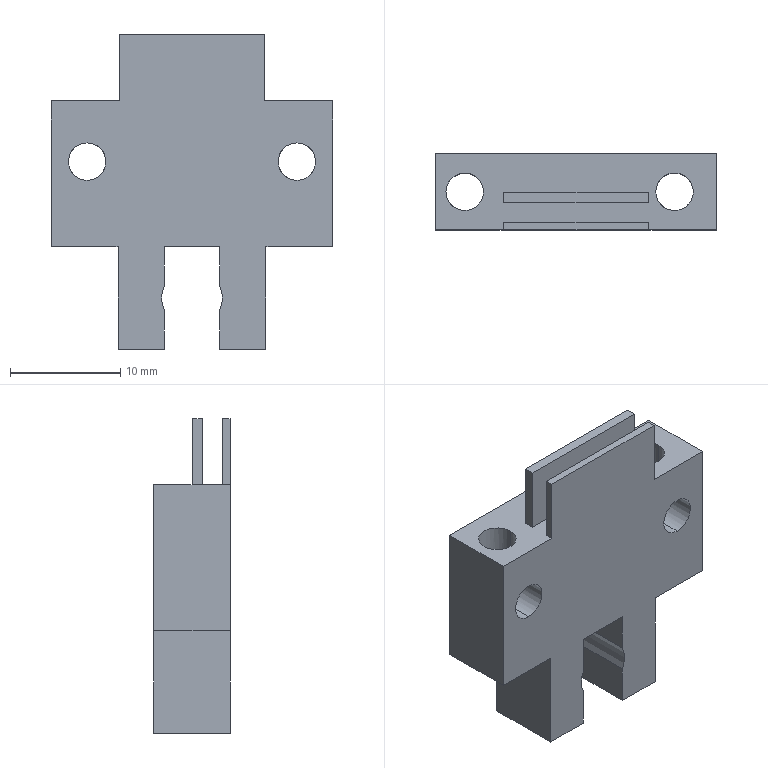Part | SolidWorks | features ICE 4, HoleWzd 2, Emboss 1, Extrusion 1 | 1 solid | 52 faces | box 25.5 x 6.9 x 28.5 mm | volume 2565 mm3 | plane 38 | cylinder 14 | commonest cylinder face diameters 3.4 x10 5 x2 5.5 x2